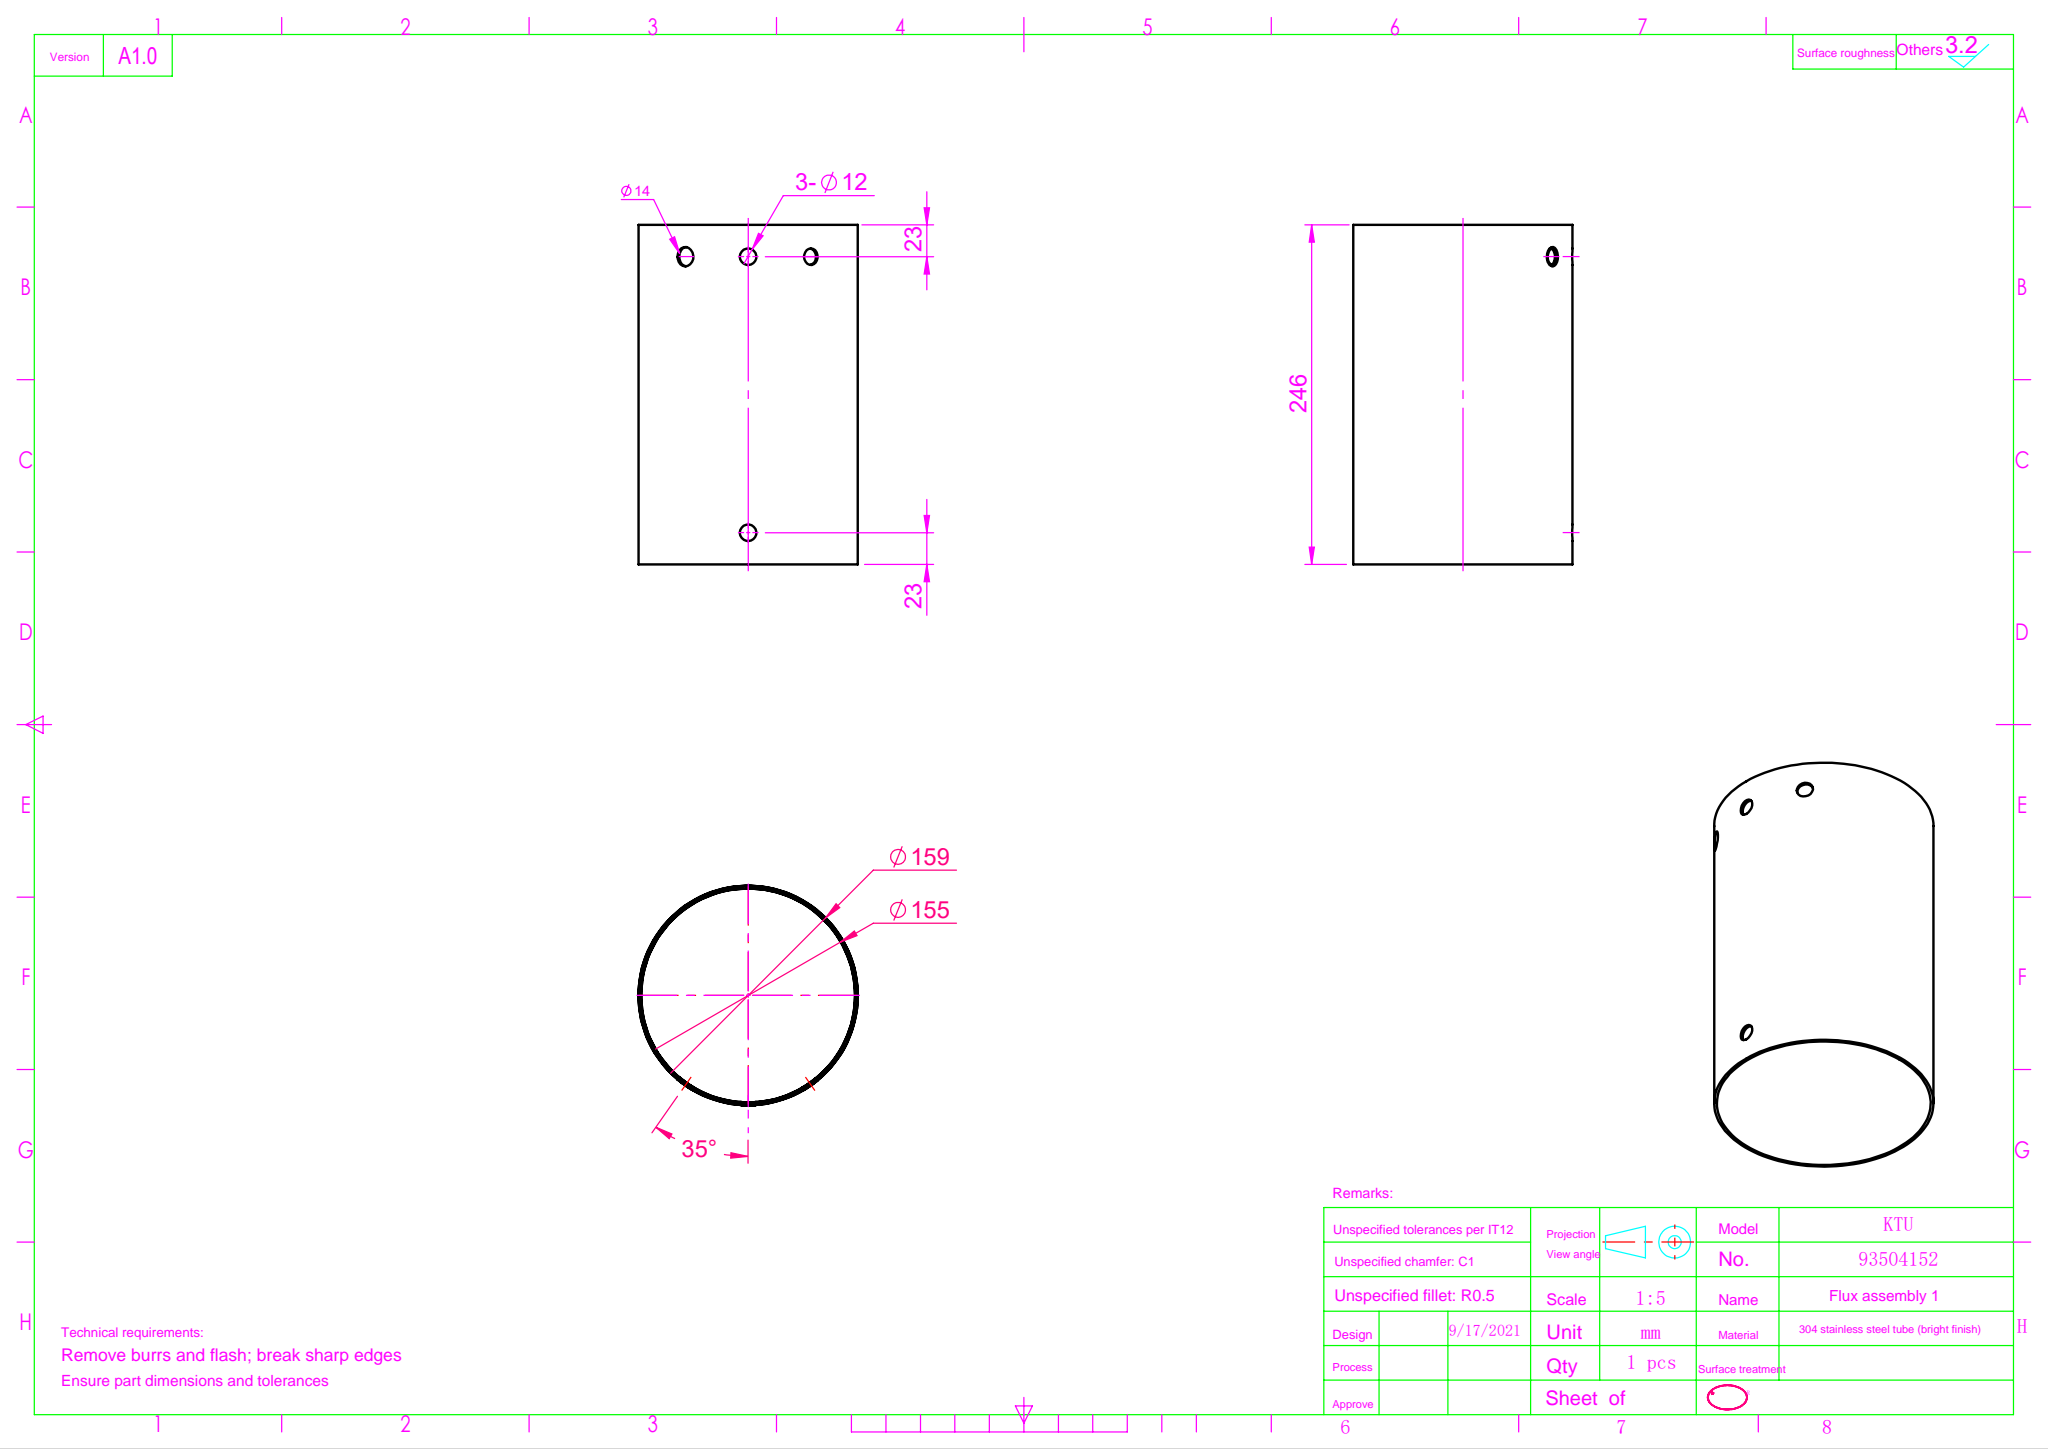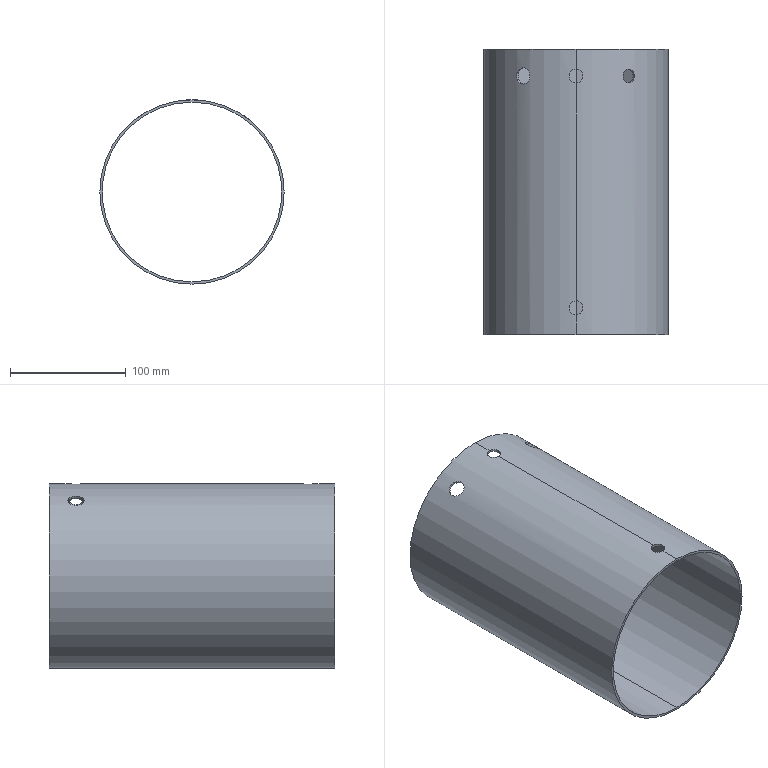Part | SolidWorks | features ICE 4, ExtruThin 1 | 1 solid | 14 faces | box 159 x 246 x 159 mm | volume 241682 mm3 | cylinder 12 | plane 2 | commonest cylinder face diameters 12 x6 14 x2 155 x2 159 x2